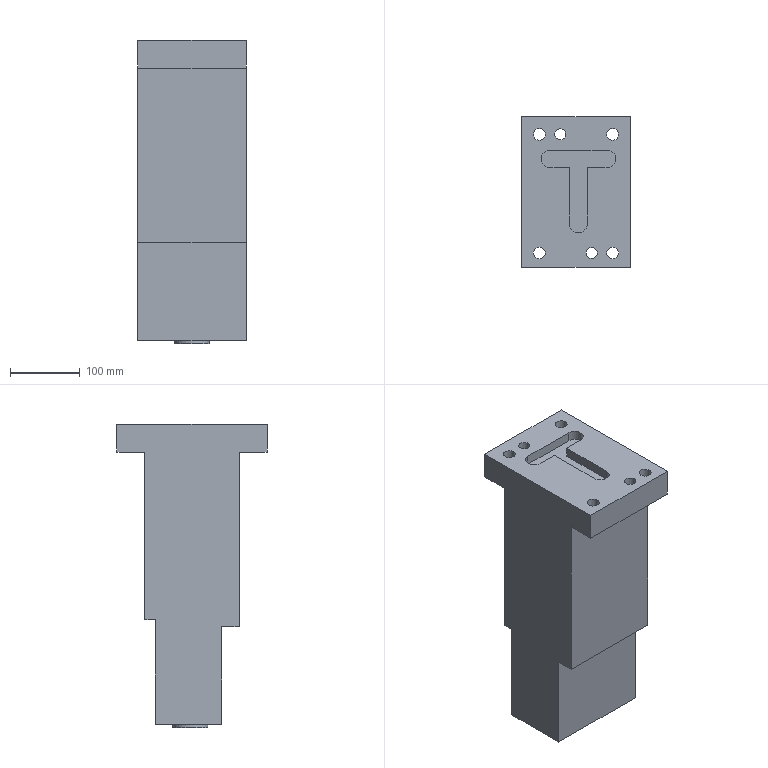Part | NX | features solid 2 | 1 solid | 41 faces | box 155 x 215 x 435 mm | volume 8461392 mm3 | plane 25 | cylinder 15 | cone 1 | commonest cylinder face diameters 25 x7 17 x4 16 x2 20 x1 50 x1
STEP:
#1=CARTESIAN_POINT('',(161.,-435.,130.));
#2=VERTEX_POINT('',#1);
#3=CARTESIAN_POINT('',(169.,-435.,130.));
#4=DIRECTION('',(0.,0.,-1.));
#5=DIRECTION('',(-1.,0.,0.));
#6=AXIS2_PLACEMENT_3D('',#3,#4,#5);
#7=CIRCLE('',#6,8.);
#8=EDGE_CURVE('',#2,#2,#7,.T.);
#9=ORIENTED_EDGE('',*,*,#8,.T.);
#10=EDGE_LOOP('',(#9));
#11=FACE_BOUND('',#10,.T.);
#12=CARTESIAN_POINT('',(206.,-605.,130.));
#13=VERTEX_POINT('',#12);
#14=CARTESIAN_POINT('',(214.,-605.,130.));
#15=DIRECTION('',(0.,0.,-1.));
#16=DIRECTION('',(-1.,0.,0.));
#17=AXIS2_PLACEMENT_3D('',#14,#15,#16);
#18=CIRCLE('',#17,8.);
#19=EDGE_CURVE('',#13,#13,#18,.T.);
#20=ORIENTED_EDGE('',*,*,#19,.T.);
#21=EDGE_LOOP('',(#20));
#22=FACE_BOUND('',#21,.T.);
#23=CARTESIAN_POINT('',(130.5,-435.,130.));
#24=VERTEX_POINT('',#23);
#25=CARTESIAN_POINT('',(139.,-435.,130.));
#26=DIRECTION('',(0.,0.,-1.));
#27=DIRECTION('',(-1.,0.,0.));
#28=AXIS2_PLACEMENT_3D('',#25,#26,#27);
#29=CIRCLE('',#28,8.5);
#30=EDGE_CURVE('',#24,#24,#29,.T.);
#31=ORIENTED_EDGE('',*,*,#30,.T.);
#32=EDGE_LOOP('',(#31));
#33=FACE_BOUND('',#32,.T.);
#34=CARTESIAN_POINT('',(235.5,-435.,130.));
#35=VERTEX_POINT('',#34);
#36=CARTESIAN_POINT('',(244.,-435.,130.));
#37=DIRECTION('',(0.,0.,-1.));
#38=DIRECTION('',(-1.,0.,0.));
#39=AXIS2_PLACEMENT_3D('',#36,#37,#38);
#40=CIRCLE('',#39,8.5);
#41=EDGE_CURVE('',#35,#35,#40,.T.);
#42=ORIENTED_EDGE('',*,*,#41,.T.);
#43=EDGE_LOOP('',(#42));
#44=FACE_BOUND('',#43,.T.);
#45=CARTESIAN_POINT('',(130.5,-605.,130.));
#46=VERTEX_POINT('',#45);
#47=CARTESIAN_POINT('',(139.,-605.,130.));
#48=DIRECTION('',(0.,0.,-1.));
#49=DIRECTION('',(-1.,0.,0.));
#50=AXIS2_PLACEMENT_3D('',#47,#48,#49);
#51=CIRCLE('',#50,8.5);
#52=EDGE_CURVE('',#46,#46,#51,.T.);
#53=ORIENTED_EDGE('',*,*,#52,.T.);
#54=EDGE_LOOP('',(#53));
#55=FACE_BOUND('',#54,.T.);
#56=CARTESIAN_POINT('',(235.5,-605.,130.));
#57=VERTEX_POINT('',#56);
#58=CARTESIAN_POINT('',(244.,-605.,130.));
#59=DIRECTION('',(0.,0.,-1.));
#60=DIRECTION('',(-1.,0.,0.));
#61=AXIS2_PLACEMENT_3D('',#58,#59,#60);
#62=CIRCLE('',#61,8.5);
#63=EDGE_CURVE('',#57,#57,#62,.T.);
#64=ORIENTED_EDGE('',*,*,#63,.T.);
#65=EDGE_LOOP('',(#64));
#66=FACE_BOUND('',#65,.T.);
#67=CARTESIAN_POINT('',(114.,-625.,130.));
#68=VERTEX_POINT('',#67);
#69=CARTESIAN_POINT('',(114.,-410.,130.));
#70=VERTEX_POINT('',#69);
#71=CARTESIAN_POINT('',(114.,-574.335,130.));
#72=DIRECTION('',(0.,1.,0.));
#73=VECTOR('',#72,1000.);
#74=LINE('',#71,#73);
#75=EDGE_CURVE('',#68,#70,#74,.T.);
#76=ORIENTED_EDGE('',*,*,#75,.F.);
#77=CARTESIAN_POINT('',(269.,-625.,130.));
#78=VERTEX_POINT('',#77);
#79=CARTESIAN_POINT('',(106.5,-625.,130.));
#80=DIRECTION('',(1.,0.,0.));
#81=VECTOR('',#80,1000.);
#82=LINE('',#79,#81);
#83=EDGE_CURVE('',#68,#78,#82,.T.);
#84=ORIENTED_EDGE('',*,*,#83,.T.);
#85=CARTESIAN_POINT('',(269.,-410.,130.));
#86=VERTEX_POINT('',#85);
#87=CARTESIAN_POINT('',(269.,-549.335,130.));
#88=DIRECTION('',(0.,1.,0.));
#89=VECTOR('',#88,1000.);
#90=LINE('',#87,#89);
#91=EDGE_CURVE('',#78,#86,#90,.T.);
#92=ORIENTED_EDGE('',*,*,#91,.T.);
#93=CARTESIAN_POINT('',(269.,-410.,130.));
#94=DIRECTION('',(1.,0.,0.));
#95=VECTOR('',#94,1000.);
#96=LINE('',#93,#95);
#97=EDGE_CURVE('',#86,#70,#96,.F.);
#98=ORIENTED_EDGE('',*,*,#97,.T.);
#99=EDGE_LOOP('',(#76,#84,#92,#98));
#100=FACE_BOUND('',#99,.T.);
#101=CARTESIAN_POINT('',(236.,-482.5,130.));
#102=VERTEX_POINT('',#101);
#103=CARTESIAN_POINT('',(207.5,-482.5,130.));
#104=VERTEX_POINT('',#103);
#105=CARTESIAN_POINT('',(106.5,-482.5,130.));
#106=DIRECTION('',(-1.,0.,0.));
#107=VECTOR('',#106,1000.);
#108=LINE('',#105,#107);
#109=EDGE_CURVE('',#102,#104,#108,.T.);
#110=ORIENTED_EDGE('',*,*,#109,.T.);
#111=CARTESIAN_POINT('',(207.5,-563.5,130.));
#112=VERTEX_POINT('',#111);
#113=CARTESIAN_POINT('',(207.5,-574.335,130.));
#114=DIRECTION('',(0.,1.,0.));
#115=VECTOR('',#114,1000.);
#116=LINE('',#113,#115);
#117=EDGE_CURVE('',#112,#104,#116,.T.);
#118=ORIENTED_EDGE('',*,*,#117,.F.);
#119=CARTESIAN_POINT('',(182.5,-563.5,130.));
#120=VERTEX_POINT('',#119);
#121=CARTESIAN_POINT('',(195.,-563.5,130.));
#122=DIRECTION('',(0.,0.,-1.));
#123=DIRECTION('',(1.,0.,0.));
#124=AXIS2_PLACEMENT_3D('',#121,#122,#123);
#125=CIRCLE('',#124,12.5);
#126=EDGE_CURVE('',#112,#120,#125,.T.);
#127=ORIENTED_EDGE('',*,*,#126,.T.);
#128=CARTESIAN_POINT('',(182.5,-482.5,130.));
#129=VERTEX_POINT('',#128);
#130=CARTESIAN_POINT('',(182.5,-574.335,130.));
#131=DIRECTION('',(0.,-1.,0.));
#132=VECTOR('',#131,1000.);
#133=LINE('',#130,#132);
#134=EDGE_CURVE('',#129,#120,#133,.T.);
#135=ORIENTED_EDGE('',*,*,#134,.F.);
#136=CARTESIAN_POINT('',(154.,-482.5,130.));
#137=VERTEX_POINT('',#136);
#138=CARTESIAN_POINT('',(106.5,-482.5,130.));
#139=DIRECTION('',(-1.,0.,0.));
#140=VECTOR('',#139,1000.);
#141=LINE('',#138,#140);
#142=EDGE_CURVE('',#129,#137,#141,.T.);
#143=ORIENTED_EDGE('',*,*,#142,.T.);
#144=CARTESIAN_POINT('',(154.,-457.5,130.));
#145=VERTEX_POINT('',#144);
#146=CARTESIAN_POINT('',(154.,-470.,130.));
#147=DIRECTION('',(0.,0.,-1.));
#148=DIRECTION('',(1.,0.,0.));
#149=AXIS2_PLACEMENT_3D('',#146,#147,#148);
#150=CIRCLE('',#149,12.5);
#151=EDGE_CURVE('',#145,#137,#150,.F.);
#152=ORIENTED_EDGE('',*,*,#151,.F.);
#153=CARTESIAN_POINT('',(236.,-457.5,130.));
#154=VERTEX_POINT('',#153);
#155=CARTESIAN_POINT('',(106.5,-457.5,130.));
#156=DIRECTION('',(-1.,0.,0.));
#157=VECTOR('',#156,1000.);
#158=LINE('',#155,#157);
#159=EDGE_CURVE('',#154,#145,#158,.T.);
#160=ORIENTED_EDGE('',*,*,#159,.F.);
#161=CARTESIAN_POINT('',(236.,-470.,130.));
#162=DIRECTION('',(0.,0.,-1.));
#163=DIRECTION('',(1.,0.,0.));
#164=AXIS2_PLACEMENT_3D('',#161,#162,#163);
#165=CIRCLE('',#164,12.5);
#166=EDGE_CURVE('',#102,#154,#165,.F.);
#167=ORIENTED_EDGE('',*,*,#166,.F.);
#168=EDGE_LOOP('',(#110,#118,#127,#135,#143,#152,#160,#167));
#169=FACE_BOUND('',#168,.T.);
#170=CARTESIAN_POINT('',(106.5,-574.335,130.));
#171=DIRECTION('',(0.,0.,1.));
#172=DIRECTION('',(0.,-1.,0.));
#173=AXIS2_PLACEMENT_3D('',#170,#171,#172);
#174=PLANE('',#173);
#175=ADVANCED_FACE('',(#11,#22,#33,#44,#55,#66,#100,#169),#174,.T.);
#176=CARTESIAN_POINT('',(256.5,-435.,90.));
#177=VERTEX_POINT('',#176);
#178=CARTESIAN_POINT('',(244.,-435.,90.));
#179=DIRECTION('',(0.,0.,1.));
#180=DIRECTION('',(1.,0.,0.));
#181=AXIS2_PLACEMENT_3D('',#178,#179,#180);
#182=CIRCLE('',#181,12.5);
#183=EDGE_CURVE('',#177,#177,#182,.T.);
#184=ORIENTED_EDGE('',*,*,#183,.T.);
#185=EDGE_LOOP('',(#184));
#186=FACE_BOUND('',#185,.T.);
#187=CARTESIAN_POINT('',(151.5,-435.,90.));
#188=VERTEX_POINT('',#187);
#189=CARTESIAN_POINT('',(139.,-435.,90.));
#190=DIRECTION('',(0.,0.,1.));
#191=DIRECTION('',(1.,0.,0.));
#192=AXIS2_PLACEMENT_3D('',#189,#190,#191);
#193=CIRCLE('',#192,12.5);
#194=EDGE_CURVE('',#188,#188,#193,.F.);
#195=ORIENTED_EDGE('',*,*,#194,.F.);
#196=EDGE_LOOP('',(#195));
#197=FACE_BOUND('',#196,.T.);
#198=CARTESIAN_POINT('',(177.,-435.,90.));
#199=VERTEX_POINT('',#198);
#200=CARTESIAN_POINT('',(169.,-435.,90.));
#201=DIRECTION('',(0.,0.,1.));
#202=DIRECTION('',(1.,0.,0.));
#203=AXIS2_PLACEMENT_3D('',#200,#201,#202);
#204=CIRCLE('',#203,8.);
#205=EDGE_CURVE('',#199,#199,#204,.F.);
#206=ORIENTED_EDGE('',*,*,#205,.F.);
#207=EDGE_LOOP('',(#206));
#208=FACE_BOUND('',#207,.T.);
#209=CARTESIAN_POINT('',(269.,-450.,90.));
#210=VERTEX_POINT('',#209);
#211=CARTESIAN_POINT('',(114.,-450.,90.));
#212=VERTEX_POINT('',#211);
#213=CARTESIAN_POINT('',(849.,-450.,90.));
#214=DIRECTION('',(-1.,0.,0.));
#215=VECTOR('',#214,1000.);
#216=LINE('',#213,#215);
#217=EDGE_CURVE('',#210,#212,#216,.T.);
#218=ORIENTED_EDGE('',*,*,#217,.T.);
#219=CARTESIAN_POINT('',(114.,-410.,90.));
#220=VERTEX_POINT('',#219);
#221=CARTESIAN_POINT('',(114.,-494.335,90.));
#222=DIRECTION('',(0.,-1.,0.));
#223=VECTOR('',#222,1000.);
#224=LINE('',#221,#223);
#225=EDGE_CURVE('',#212,#220,#224,.F.);
#226=ORIENTED_EDGE('',*,*,#225,.T.);
#227=CARTESIAN_POINT('',(269.,-410.,90.));
#228=VERTEX_POINT('',#227);
#229=CARTESIAN_POINT('',(269.,-410.,90.));
#230=DIRECTION('',(-1.,0.,0.));
#231=VECTOR('',#230,1000.);
#232=LINE('',#229,#231);
#233=EDGE_CURVE('',#228,#220,#232,.T.);
#234=ORIENTED_EDGE('',*,*,#233,.F.);
#235=CARTESIAN_POINT('',(269.,-549.335,90.));
#236=DIRECTION('',(0.,-1.,0.));
#237=VECTOR('',#236,1000.);
#238=LINE('',#235,#237);
#239=EDGE_CURVE('',#210,#228,#238,.F.);
#240=ORIENTED_EDGE('',*,*,#239,.F.);
#241=EDGE_LOOP('',(#218,#226,#234,#240));
#242=FACE_BOUND('',#241,.T.);
#243=CARTESIAN_POINT('',(269.,-494.335,90.));
#244=DIRECTION('',(0.,0.,-1.));
#245=DIRECTION('',(-1.,0.,0.));
#246=AXIS2_PLACEMENT_3D('',#243,#244,#245);
#247=PLANE('',#246);
#248=ADVANCED_FACE('',(#186,#197,#208,#242),#247,.T.);
#249=CARTESIAN_POINT('',(256.5,-605.,90.));
#250=VERTEX_POINT('',#249);
#251=CARTESIAN_POINT('',(244.,-605.,90.));
#252=DIRECTION('',(0.,0.,1.));
#253=DIRECTION('',(1.,0.,0.));
#254=AXIS2_PLACEMENT_3D('',#251,#252,#253);
#255=CIRCLE('',#254,12.5);
#256=EDGE_CURVE('',#250,#250,#255,.F.);
#257=ORIENTED_EDGE('',*,*,#256,.F.);
#258=EDGE_LOOP('',(#257));
#259=FACE_BOUND('',#258,.T.);
#260=CARTESIAN_POINT('',(151.5,-605.,90.));
#261=VERTEX_POINT('',#260);
#262=CARTESIAN_POINT('',(139.,-605.,90.));
#263=DIRECTION('',(0.,0.,1.));
#264=DIRECTION('',(1.,0.,0.));
#265=AXIS2_PLACEMENT_3D('',#262,#263,#264);
#266=CIRCLE('',#265,12.5);
#267=EDGE_CURVE('',#261,#261,#266,.F.);
#268=ORIENTED_EDGE('',*,*,#267,.F.);
#269=EDGE_LOOP('',(#268));
#270=FACE_BOUND('',#269,.T.);
#271=CARTESIAN_POINT('',(222.,-605.,90.));
#272=VERTEX_POINT('',#271);
#273=CARTESIAN_POINT('',(214.,-605.,90.));
#274=DIRECTION('',(0.,0.,1.));
#275=DIRECTION('',(1.,0.,0.));
#276=AXIS2_PLACEMENT_3D('',#273,#274,#275);
#277=CIRCLE('',#276,8.);
#278=EDGE_CURVE('',#272,#272,#277,.F.);
#279=ORIENTED_EDGE('',*,*,#278,.F.);
#280=EDGE_LOOP('',(#279));
#281=FACE_BOUND('',#280,.T.);
#282=CARTESIAN_POINT('',(114.,-585.,90.));
#283=VERTEX_POINT('',#282);
#284=CARTESIAN_POINT('',(269.,-585.,90.));
#285=VERTEX_POINT('',#284);
#286=CARTESIAN_POINT('',(269.,-585.,90.));
#287=DIRECTION('',(1.,0.,0.));
#288=VECTOR('',#287,1000.);
#289=LINE('',#286,#288);
#290=EDGE_CURVE('',#283,#285,#289,.T.);
#291=ORIENTED_EDGE('',*,*,#290,.T.);
#292=CARTESIAN_POINT('',(269.,-625.,90.));
#293=VERTEX_POINT('',#292);
#294=CARTESIAN_POINT('',(269.,-489.335,90.));
#295=DIRECTION('',(0.,1.,0.));
#296=VECTOR('',#295,1000.);
#297=LINE('',#294,#296);
#298=EDGE_CURVE('',#285,#293,#297,.F.);
#299=ORIENTED_EDGE('',*,*,#298,.T.);
#300=CARTESIAN_POINT('',(114.,-625.,90.));
#301=VERTEX_POINT('',#300);
#302=CARTESIAN_POINT('',(269.,-625.,90.));
#303=DIRECTION('',(-1.,0.,0.));
#304=VECTOR('',#303,1000.);
#305=LINE('',#302,#304);
#306=EDGE_CURVE('',#301,#293,#305,.F.);
#307=ORIENTED_EDGE('',*,*,#306,.F.);
#308=CARTESIAN_POINT('',(114.,-489.335,90.));
#309=DIRECTION('',(0.,-1.,0.));
#310=VECTOR('',#309,1000.);
#311=LINE('',#308,#310);
#312=EDGE_CURVE('',#301,#283,#311,.F.);
#313=ORIENTED_EDGE('',*,*,#312,.T.);
#314=EDGE_LOOP('',(#291,#299,#307,#313));
#315=FACE_BOUND('',#314,.T.);
#316=CARTESIAN_POINT('',(269.,-489.335,90.));
#317=DIRECTION('',(0.,0.,-1.));
#318=DIRECTION('',(-1.,0.,0.));
#319=AXIS2_PLACEMENT_3D('',#316,#317,#318);
#320=PLANE('',#319);
#321=ADVANCED_FACE('',(#259,#270,#281,#315),#320,.T.);
#322=ORIENTED_EDGE('',*,*,#312,.F.);
#323=CARTESIAN_POINT('',(114.,-625.,215.));
#324=DIRECTION('',(0.,0.,-1.));
#325=VECTOR('',#324,1000.);
#326=LINE('',#323,#325);
#327=EDGE_CURVE('',#68,#301,#326,.T.);
#328=ORIENTED_EDGE('',*,*,#327,.F.);
#329=ORIENTED_EDGE('',*,*,#75,.T.);
#330=CARTESIAN_POINT('',(114.,-410.,190.));
#331=DIRECTION('',(0.,0.,1.));
#332=VECTOR('',#331,1000.);
#333=LINE('',#330,#332);
#334=EDGE_CURVE('',#220,#70,#333,.T.);
#335=ORIENTED_EDGE('',*,*,#334,.F.);
#336=ORIENTED_EDGE('',*,*,#225,.F.);
#337=CARTESIAN_POINT('',(114.,-450.,-150.));
#338=VERTEX_POINT('',#337);
#339=CARTESIAN_POINT('',(114.,-450.,-43.));
#340=DIRECTION('',(0.,0.,-1.));
#341=VECTOR('',#340,1000.);
#342=LINE('',#339,#341);
#343=EDGE_CURVE('',#212,#338,#342,.T.);
#344=ORIENTED_EDGE('',*,*,#343,.T.);
#345=CARTESIAN_POINT('',(114.,-465.,-150.));
#346=VERTEX_POINT('',#345);
#347=CARTESIAN_POINT('',(114.,-559.335,-150.));
#348=DIRECTION('',(0.,1.,0.));
#349=VECTOR('',#348,1000.);
#350=LINE('',#347,#349);
#351=EDGE_CURVE('',#338,#346,#350,.F.);
#352=ORIENTED_EDGE('',*,*,#351,.T.);
#353=CARTESIAN_POINT('',(114.,-465.,-300.));
#354=VERTEX_POINT('',#353);
#355=CARTESIAN_POINT('',(114.,-465.,10.));
#356=DIRECTION('',(0.,0.,-1.));
#357=VECTOR('',#356,1000.);
#358=LINE('',#355,#357);
#359=EDGE_CURVE('',#346,#354,#358,.T.);
#360=ORIENTED_EDGE('',*,*,#359,.T.);
#361=CARTESIAN_POINT('',(114.,-560.,-300.));
#362=VERTEX_POINT('',#361);
#363=CARTESIAN_POINT('',(114.,-574.793,-300.));
#364=DIRECTION('',(0.,-1.,0.));
#365=VECTOR('',#364,1000.);
#366=LINE('',#363,#365);
#367=EDGE_CURVE('',#354,#362,#366,.T.);
#368=ORIENTED_EDGE('',*,*,#367,.T.);
#369=CARTESIAN_POINT('',(114.,-560.,-160.));
#370=VERTEX_POINT('',#369);
#371=CARTESIAN_POINT('',(114.,-560.,-105.));
#372=DIRECTION('',(0.,0.,-1.));
#373=VECTOR('',#372,1000.);
#374=LINE('',#371,#373);
#375=EDGE_CURVE('',#370,#362,#374,.T.);
#376=ORIENTED_EDGE('',*,*,#375,.F.);
#377=CARTESIAN_POINT('',(114.,-585.,-160.));
#378=VERTEX_POINT('',#377);
#379=CARTESIAN_POINT('',(114.,-564.335,-160.));
#380=DIRECTION('',(0.,1.,0.));
#381=VECTOR('',#380,1000.);
#382=LINE('',#379,#381);
#383=EDGE_CURVE('',#370,#378,#382,.F.);
#384=ORIENTED_EDGE('',*,*,#383,.T.);
#385=CARTESIAN_POINT('',(114.,-585.,-110.));
#386=DIRECTION('',(0.,0.,-1.));
#387=VECTOR('',#386,1000.);
#388=LINE('',#385,#387);
#389=EDGE_CURVE('',#378,#283,#388,.F.);
#390=ORIENTED_EDGE('',*,*,#389,.T.);
#391=EDGE_LOOP('',(#322,#328,#329,#335,#336,#344,#352,#360,#368,#376,#384,#390));
#392=FACE_BOUND('',#391,.T.);
#393=CARTESIAN_POINT('',(114.,-559.335,-105.));
#394=DIRECTION('',(-1.,0.,0.));
#395=DIRECTION('',(0.,1.,0.));
#396=AXIS2_PLACEMENT_3D('',#393,#394,#395);
#397=PLANE('',#396);
#398=ADVANCED_FACE('',(#392),#397,.T.);
#399=ORIENTED_EDGE('',*,*,#91,.F.);
#400=CARTESIAN_POINT('',(269.,-625.,215.));
#401=DIRECTION('',(0.,0.,1.));
#402=VECTOR('',#401,1000.);
#403=LINE('',#400,#402);
#404=EDGE_CURVE('',#293,#78,#403,.T.);
#405=ORIENTED_EDGE('',*,*,#404,.F.);
#406=ORIENTED_EDGE('',*,*,#298,.F.);
#407=CARTESIAN_POINT('',(269.,-585.,-160.));
#408=VERTEX_POINT('',#407);
#409=CARTESIAN_POINT('',(269.,-585.,-40.));
#410=DIRECTION('',(0.,0.,-1.));
#411=VECTOR('',#410,1000.);
#412=LINE('',#409,#411);
#413=EDGE_CURVE('',#408,#285,#412,.F.);
#414=ORIENTED_EDGE('',*,*,#413,.F.);
#415=CARTESIAN_POINT('',(269.,-560.,-160.));
#416=VERTEX_POINT('',#415);
#417=CARTESIAN_POINT('',(269.,-549.335,-160.));
#418=DIRECTION('',(0.,1.,0.));
#419=VECTOR('',#418,1000.);
#420=LINE('',#417,#419);
#421=EDGE_CURVE('',#416,#408,#420,.F.);
#422=ORIENTED_EDGE('',*,*,#421,.F.);
#423=CARTESIAN_POINT('',(269.,-560.,-300.));
#424=VERTEX_POINT('',#423);
#425=CARTESIAN_POINT('',(269.,-560.,-50.));
#426=DIRECTION('',(0.,0.,-1.));
#427=VECTOR('',#426,1000.);
#428=LINE('',#425,#427);
#429=EDGE_CURVE('',#416,#424,#428,.T.);
#430=ORIENTED_EDGE('',*,*,#429,.T.);
#431=CARTESIAN_POINT('',(269.,-465.,-300.));
#432=VERTEX_POINT('',#431);
#433=CARTESIAN_POINT('',(269.,-549.335,-300.));
#434=DIRECTION('',(0.,-1.,0.));
#435=VECTOR('',#434,1000.);
#436=LINE('',#433,#435);
#437=EDGE_CURVE('',#432,#424,#436,.T.);
#438=ORIENTED_EDGE('',*,*,#437,.F.);
#439=CARTESIAN_POINT('',(269.,-465.,-150.));
#440=VERTEX_POINT('',#439);
#441=CARTESIAN_POINT('',(269.,-465.,-105.));
#442=DIRECTION('',(0.,0.,-1.));
#443=VECTOR('',#442,1000.);
#444=LINE('',#441,#443);
#445=EDGE_CURVE('',#440,#432,#444,.T.);
#446=ORIENTED_EDGE('',*,*,#445,.F.);
#447=CARTESIAN_POINT('',(269.,-450.,-150.));
#448=VERTEX_POINT('',#447);
#449=CARTESIAN_POINT('',(269.,-455.,-150.));
#450=DIRECTION('',(0.,1.,0.));
#451=VECTOR('',#450,1000.);
#452=LINE('',#449,#451);
#453=EDGE_CURVE('',#448,#440,#452,.F.);
#454=ORIENTED_EDGE('',*,*,#453,.F.);
#455=CARTESIAN_POINT('',(269.,-450.,-105.));
#456=DIRECTION('',(0.,0.,-1.));
#457=VECTOR('',#456,1000.);
#458=LINE('',#455,#457);
#459=EDGE_CURVE('',#210,#448,#458,.T.);
#460=ORIENTED_EDGE('',*,*,#459,.F.);
#461=ORIENTED_EDGE('',*,*,#239,.T.);
#462=CARTESIAN_POINT('',(269.,-410.,-105.));
#463=DIRECTION('',(0.,0.,1.));
#464=VECTOR('',#463,1000.);
#465=LINE('',#462,#464);
#466=EDGE_CURVE('',#86,#228,#465,.F.);
#467=ORIENTED_EDGE('',*,*,#466,.F.);
#468=EDGE_LOOP('',(#399,#405,#406,#414,#422,#430,#438,#446,#454,#460,#461,#467));
#469=FACE_BOUND('',#468,.T.);
#470=CARTESIAN_POINT('',(269.,-549.335,-105.));
#471=DIRECTION('',(1.,0.,0.));
#472=DIRECTION('',(0.,-1.,0.));
#473=AXIS2_PLACEMENT_3D('',#470,#471,#472);
#474=PLANE('',#473);
#475=ADVANCED_FACE('',(#469),#474,.T.);
#476=ORIENTED_EDGE('',*,*,#404,.T.);
#477=ORIENTED_EDGE('',*,*,#83,.F.);
#478=ORIENTED_EDGE('',*,*,#327,.T.);
#479=ORIENTED_EDGE('',*,*,#306,.T.);
#480=EDGE_LOOP('',(#476,#477,#478,#479));
#481=FACE_BOUND('',#480,.T.);
#482=CARTESIAN_POINT('',(106.5,-625.,115.));
#483=DIRECTION('',(0.,1.,0.));
#484=DIRECTION('',(0.,0.,-1.));
#485=AXIS2_PLACEMENT_3D('',#482,#483,#484);
#486=PLANE('',#485);
#487=ADVANCED_FACE('',(#481),#486,.F.);
#488=ORIENTED_EDGE('',*,*,#233,.T.);
#489=ORIENTED_EDGE('',*,*,#334,.T.);
#490=ORIENTED_EDGE('',*,*,#97,.F.);
#491=ORIENTED_EDGE('',*,*,#466,.T.);
#492=EDGE_LOOP('',(#488,#489,#490,#491));
#493=FACE_BOUND('',#492,.T.);
#494=CARTESIAN_POINT('',(269.,-410.,90.));
#495=DIRECTION('',(0.,-1.,0.));
#496=DIRECTION('',(0.,0.,-1.));
#497=AXIS2_PLACEMENT_3D('',#494,#495,#496);
#498=PLANE('',#497);
#499=ADVANCED_FACE('',(#493),#498,.F.);
#500=ORIENTED_EDGE('',*,*,#63,.F.);
#501=EDGE_LOOP('',(#500));
#502=FACE_BOUND('',#501,.T.);
#503=CARTESIAN_POINT('',(252.5,-605.,110.));
#504=VERTEX_POINT('',#503);
#505=CARTESIAN_POINT('',(244.,-605.,110.));
#506=DIRECTION('',(0.,0.,-1.));
#507=DIRECTION('',(1.,0.,0.));
#508=AXIS2_PLACEMENT_3D('',#505,#506,#507);
#509=CIRCLE('',#508,8.5);
#510=EDGE_CURVE('',#504,#504,#509,.T.);
#511=ORIENTED_EDGE('',*,*,#510,.T.);
#512=EDGE_LOOP('',(#511));
#513=FACE_BOUND('',#512,.T.);
#514=CARTESIAN_POINT('',(244.,-605.,130.));
#515=DIRECTION('',(0.,0.,1.));
#516=DIRECTION('',(-1.,0.,0.));
#517=AXIS2_PLACEMENT_3D('',#514,#515,#516);
#518=CYLINDRICAL_SURFACE('',#517,8.5);
#519=ADVANCED_FACE('',(#502,#513),#518,.F.);
#520=ORIENTED_EDGE('',*,*,#510,.F.);
#521=EDGE_LOOP('',(#520));
#522=FACE_BOUND('',#521,.T.);
#523=CARTESIAN_POINT('',(256.5,-605.,110.));
#524=VERTEX_POINT('',#523);
#525=CARTESIAN_POINT('',(244.,-605.,110.));
#526=DIRECTION('',(0.,0.,-1.));
#527=DIRECTION('',(1.,0.,0.));
#528=AXIS2_PLACEMENT_3D('',#525,#526,#527);
#529=CIRCLE('',#528,12.5);
#530=EDGE_CURVE('',#524,#524,#529,.T.);
#531=ORIENTED_EDGE('',*,*,#530,.T.);
#532=EDGE_LOOP('',(#531));
#533=FACE_BOUND('',#532,.T.);
#534=CARTESIAN_POINT('',(139.,-435.,110.));
#535=DIRECTION('',(0.,0.,1.));
#536=DIRECTION('',(-1.,0.,0.));
#537=AXIS2_PLACEMENT_3D('',#534,#535,#536);
#538=PLANE('',#537);
#539=ADVANCED_FACE('',(#522,#533),#538,.F.);
#540=ORIENTED_EDGE('',*,*,#530,.F.);
#541=EDGE_LOOP('',(#540));
#542=FACE_BOUND('',#541,.T.);
#543=ORIENTED_EDGE('',*,*,#256,.T.);
#544=EDGE_LOOP('',(#543));
#545=FACE_BOUND('',#544,.T.);
#546=CARTESIAN_POINT('',(244.,-605.,80.));
#547=DIRECTION('',(0.,0.,1.));
#548=DIRECTION('',(-1.,0.,0.));
#549=AXIS2_PLACEMENT_3D('',#546,#547,#548);
#550=CYLINDRICAL_SURFACE('',#549,12.5);
#551=ADVANCED_FACE('',(#542,#545),#550,.F.);
#552=ORIENTED_EDGE('',*,*,#52,.F.);
#553=EDGE_LOOP('',(#552));
#554=FACE_BOUND('',#553,.T.);
#555=CARTESIAN_POINT('',(147.5,-605.,110.));
#556=VERTEX_POINT('',#555);
#557=CARTESIAN_POINT('',(139.,-605.,110.));
#558=DIRECTION('',(0.,0.,-1.));
#559=DIRECTION('',(1.,0.,0.));
#560=AXIS2_PLACEMENT_3D('',#557,#558,#559);
#561=CIRCLE('',#560,8.5);
#562=EDGE_CURVE('',#556,#556,#561,.T.);
#563=ORIENTED_EDGE('',*,*,#562,.T.);
#564=EDGE_LOOP('',(#563));
#565=FACE_BOUND('',#564,.T.);
#566=CARTESIAN_POINT('',(139.,-605.,130.));
#567=DIRECTION('',(0.,0.,1.));
#568=DIRECTION('',(-1.,0.,0.));
#569=AXIS2_PLACEMENT_3D('',#566,#567,#568);
#570=CYLINDRICAL_SURFACE('',#569,8.5);
#571=ADVANCED_FACE('',(#554,#565),#570,.F.);
#572=ORIENTED_EDGE('',*,*,#562,.F.);
#573=EDGE_LOOP('',(#572));
#574=FACE_BOUND('',#573,.T.);
#575=CARTESIAN_POINT('',(151.5,-605.,110.));
#576=VERTEX_POINT('',#575);
#577=CARTESIAN_POINT('',(139.,-605.,110.));
#578=DIRECTION('',(0.,0.,-1.));
#579=DIRECTION('',(1.,0.,0.));
#580=AXIS2_PLACEMENT_3D('',#577,#578,#579);
#581=CIRCLE('',#580,12.5);
#582=EDGE_CURVE('',#576,#576,#581,.T.);
#583=ORIENTED_EDGE('',*,*,#582,.T.);
#584=EDGE_LOOP('',(#583));
#585=FACE_BOUND('',#584,.T.);
#586=CARTESIAN_POINT('',(139.,-435.,110.));
#587=DIRECTION('',(0.,0.,1.));
#588=DIRECTION('',(-1.,0.,0.));
#589=AXIS2_PLACEMENT_3D('',#586,#587,#588);
#590=PLANE('',#589);
#591=ADVANCED_FACE('',(#574,#585),#590,.F.);
#592=ORIENTED_EDGE('',*,*,#582,.F.);
#593=EDGE_LOOP('',(#592));
#594=FACE_BOUND('',#593,.T.);
#595=ORIENTED_EDGE('',*,*,#267,.T.);
#596=EDGE_LOOP('',(#595));
#597=FACE_BOUND('',#596,.T.);
#598=CARTESIAN_POINT('',(139.,-605.,80.));
#599=DIRECTION('',(0.,0.,1.));
#600=DIRECTION('',(-1.,0.,0.));
#601=AXIS2_PLACEMENT_3D('',#598,#599,#600);
#602=CYLINDRICAL_SURFACE('',#601,12.5);
#603=ADVANCED_FACE('',(#594,#597),#602,.F.);
#604=ORIENTED_EDGE('',*,*,#41,.F.);
#605=EDGE_LOOP('',(#604));
#606=FACE_BOUND('',#605,.T.);
#607=CARTESIAN_POINT('',(252.5,-435.,110.));
#608=VERTEX_POINT('',#607);
#609=CARTESIAN_POINT('',(244.,-435.,110.));
#610=DIRECTION('',(0.,0.,-1.));
#611=DIRECTION('',(1.,0.,0.));
#612=AXIS2_PLACEMENT_3D('',#609,#610,#611);
#613=CIRCLE('',#612,8.5);
#614=EDGE_CURVE('',#608,#608,#613,.T.);
#615=ORIENTED_EDGE('',*,*,#614,.T.);
#616=EDGE_LOOP('',(#615));
#617=FACE_BOUND('',#616,.T.);
#618=CARTESIAN_POINT('',(244.,-435.,140.));
#619=DIRECTION('',(0.,0.,1.));
#620=DIRECTION('',(-1.,0.,0.));
#621=AXIS2_PLACEMENT_3D('',#618,#619,#620);
#622=CYLINDRICAL_SURFACE('',#621,8.5);
#623=ADVANCED_FACE('',(#606,#617),#622,.F.);
#624=ORIENTED_EDGE('',*,*,#614,.F.);
#625=EDGE_LOOP('',(#624));
#626=FACE_BOUND('',#625,.T.);
#627=CARTESIAN_POINT('',(256.5,-435.,110.));
#628=VERTEX_POINT('',#627);
#629=CARTESIAN_POINT('',(244.,-435.,110.));
#630=DIRECTION('',(0.,0.,-1.));
#631=DIRECTION('',(1.,0.,0.));
#632=AXIS2_PLACEMENT_3D('',#629,#630,#631);
#633=CIRCLE('',#632,12.5);
#634=EDGE_CURVE('',#628,#628,#633,.T.);
#635=ORIENTED_EDGE('',*,*,#634,.T.);
#636=EDGE_LOOP('',(#635));
#637=FACE_BOUND('',#636,.T.);
#638=CARTESIAN_POINT('',(139.,-435.,110.));
#639=DIRECTION('',(0.,0.,1.));
#640=DIRECTION('',(-1.,0.,0.));
#641=AXIS2_PLACEMENT_3D('',#638,#639,#640);
#642=PLANE('',#641);
#643=ADVANCED_FACE('',(#626,#637),#642,.F.);
#644=ORIENTED_EDGE('',*,*,#634,.F.);
#645=EDGE_LOOP('',(#644));
#646=FACE_BOUND('',#645,.T.);
#647=ORIENTED_EDGE('',*,*,#183,.F.);
#648=EDGE_LOOP('',(#647));
#649=FACE_BOUND('',#648,.T.);
#650=CARTESIAN_POINT('',(244.,-435.,90.));
#651=DIRECTION('',(0.,0.,1.));
#652=DIRECTION('',(-1.,0.,0.));
#653=AXIS2_PLACEMENT_3D('',#650,#651,#652);
#654=CYLINDRICAL_SURFACE('',#653,12.5);
#655=ADVANCED_FACE('',(#646,#649),#654,.F.);
#656=ORIENTED_EDGE('',*,*,#30,.F.);
#657=EDGE_LOOP('',(#656));
#658=FACE_BOUND('',#657,.T.);
#659=CARTESIAN_POINT('',(130.5,-435.,110.));
#660=VERTEX_POINT('',#659);
#661=CARTESIAN_POINT('',(139.,-435.,110.));
#662=DIRECTION('',(0.,0.,-1.));
#663=DIRECTION('',(-1.,0.,0.));
#664=AXIS2_PLACEMENT_3D('',#661,#662,#663);
#665=CIRCLE('',#664,8.5);
#666=EDGE_CURVE('',#660,#660,#665,.T.);
#667=ORIENTED_EDGE('',*,*,#666,.T.);
#668=EDGE_LOOP('',(#667));
#669=FACE_BOUND('',#668,.T.);
#670=CARTESIAN_POINT('',(139.,-435.,140.));
#671=DIRECTION('',(0.,0.,1.));
#672=DIRECTION('',(-1.,0.,0.));
#673=AXIS2_PLACEMENT_3D('',#670,#671,#672);
#674=CYLINDRICAL_SURFACE('',#673,8.5);
#675=ADVANCED_FACE('',(#658,#669),#674,.F.);
#676=ORIENTED_EDGE('',*,*,#666,.F.);
#677=EDGE_LOOP('',(#676));
#678=FACE_BOUND('',#677,.T.);
#679=CARTESIAN_POINT('',(126.5,-435.,110.));
#680=VERTEX_POINT('',#679);
#681=CARTESIAN_POINT('',(139.,-435.,110.));
#682=DIRECTION('',(0.,0.,-1.));
#683=DIRECTION('',(-1.,0.,0.));
#684=AXIS2_PLACEMENT_3D('',#681,#682,#683);
#685=CIRCLE('',#684,12.5);
#686=EDGE_CURVE('',#680,#680,#685,.T.);
#687=ORIENTED_EDGE('',*,*,#686,.T.);
#688=EDGE_LOOP('',(#687));
#689=FACE_BOUND('',#688,.T.);
#690=CARTESIAN_POINT('',(139.,-435.,110.));
#691=DIRECTION('',(0.,0.,1.));
#692=DIRECTION('',(-1.,0.,0.));
#693=AXIS2_PLACEMENT_3D('',#690,#691,#692);
#694=PLANE('',#693);
#695=ADVANCED_FACE('',(#678,#689),#694,.F.);
#696=ORIENTED_EDGE('',*,*,#686,.F.);
#697=EDGE_LOOP('',(#696));
#698=FACE_BOUND('',#697,.T.);
#699=ORIENTED_EDGE('',*,*,#194,.T.);
#700=EDGE_LOOP('',(#699));
#701=FACE_BOUND('',#700,.T.);
#702=CARTESIAN_POINT('',(139.,-435.,90.));
#703=DIRECTION('',(0.,0.,1.));
#704=DIRECTION('',(-1.,0.,0.));
#705=AXIS2_PLACEMENT_3D('',#702,#703,#704);
#706=CYLINDRICAL_SURFACE('',#705,12.5);
#707=ADVANCED_FACE('',(#698,#701),#706,.F.);
#708=ORIENTED_EDGE('',*,*,#19,.F.);
#709=EDGE_LOOP('',(#708));
#710=FACE_BOUND('',#709,.T.);
#711=ORIENTED_EDGE('',*,*,#278,.T.);
#712=EDGE_LOOP('',(#711));
#713=FACE_BOUND('',#712,.T.);
#714=CARTESIAN_POINT('',(214.,-605.,80.));
#715=DIRECTION('',(0.,0.,1.));
#716=DIRECTION('',(-1.,0.,0.));
#717=AXIS2_PLACEMENT_3D('',#714,#715,#716);
#718=CYLINDRICAL_SURFACE('',#717,8.);
#719=ADVANCED_FACE('',(#710,#713),#718,.F.);
#720=ORIENTED_EDGE('',*,*,#8,.F.);
#721=EDGE_LOOP('',(#720));
#722=FACE_BOUND('',#721,.T.);
#723=ORIENTED_EDGE('',*,*,#205,.T.);
#724=EDGE_LOOP('',(#723));
#725=FACE_BOUND('',#724,.T.);
#726=CARTESIAN_POINT('',(169.,-435.,90.));
#727=DIRECTION('',(0.,0.,1.));
#728=DIRECTION('',(-1.,0.,0.));
#729=AXIS2_PLACEMENT_3D('',#726,#727,#728);
#730=CYLINDRICAL_SURFACE('',#729,8.);
#731=ADVANCED_FACE('',(#722,#725),#730,.F.);
#732=ORIENTED_EDGE('',*,*,#459,.T.);
#733=CARTESIAN_POINT('',(229.,-450.,-150.));
#734=DIRECTION('',(-1.,0.,0.));
#735=VECTOR('',#734,1000.);
#736=LINE('',#733,#735);
#737=EDGE_CURVE('',#338,#448,#736,.F.);
#738=ORIENTED_EDGE('',*,*,#737,.F.);
#739=ORIENTED_EDGE('',*,*,#343,.F.);
#740=ORIENTED_EDGE('',*,*,#217,.F.);
#741=EDGE_LOOP('',(#732,#738,#739,#740));
#742=FACE_BOUND('',#741,.T.);
#743=CARTESIAN_POINT('',(688.5,-450.,-143.));
#744=DIRECTION('',(0.,1.,0.));
#745=DIRECTION('',(1.,0.,0.));
#746=AXIS2_PLACEMENT_3D('',#743,#744,#745);
#747=PLANE('',#746);
#748=ADVANCED_FACE('',(#742),#747,.T.);
#749=CARTESIAN_POINT('',(166.5,-515.,-300.));
#750=VERTEX_POINT('',#749);
#751=CARTESIAN_POINT('',(191.5,-515.,-300.));
#752=DIRECTION('',(0.,0.,1.));
#753=DIRECTION('',(-1.,0.,0.));
#754=AXIS2_PLACEMENT_3D('',#751,#752,#753);
#755=CIRCLE('',#754,25.);
#756=EDGE_CURVE('',#750,#750,#755,.T.);
#757=ORIENTED_EDGE('',*,*,#756,.T.);
#758=EDGE_LOOP('',(#757));
#759=FACE_BOUND('',#758,.T.);
#760=CARTESIAN_POINT('',(229.,-560.,-300.));
#761=DIRECTION('',(1.,0.,0.));
#762=VECTOR('',#761,1000.);
#763=LINE('',#760,#762);
#764=EDGE_CURVE('',#362,#424,#763,.T.);
#765=ORIENTED_EDGE('',*,*,#764,.F.);
#766=ORIENTED_EDGE('',*,*,#367,.F.);
#767=CARTESIAN_POINT('',(382.,-465.,-300.));
#768=DIRECTION('',(1.,0.,0.));
#769=VECTOR('',#768,1000.);
#770=LINE('',#767,#769);
#771=EDGE_CURVE('',#354,#432,#770,.T.);
#772=ORIENTED_EDGE('',*,*,#771,.T.);
#773=ORIENTED_EDGE('',*,*,#437,.T.);
#774=EDGE_LOOP('',(#765,#766,#772,#773));
#775=FACE_BOUND('',#774,.T.);
#776=CARTESIAN_POINT('',(229.,-574.793,-300.));
#777=DIRECTION('',(0.,0.,-1.));
#778=DIRECTION('',(-1.,0.,0.));
#779=AXIS2_PLACEMENT_3D('',#776,#777,#778);
#780=PLANE('',#779);
#781=ADVANCED_FACE('',(#759,#775),#780,.T.);
#782=ORIENTED_EDGE('',*,*,#290,.F.);
#783=ORIENTED_EDGE('',*,*,#389,.F.);
#784=CARTESIAN_POINT('',(686.5,-585.,-160.));
#785=DIRECTION('',(1.,0.,0.));
#786=VECTOR('',#785,1000.);
#787=LINE('',#784,#786);
#788=EDGE_CURVE('',#378,#408,#787,.T.);
#789=ORIENTED_EDGE('',*,*,#788,.T.);
#790=ORIENTED_EDGE('',*,*,#413,.T.);
#791=EDGE_LOOP('',(#782,#783,#789,#790));
#792=FACE_BOUND('',#791,.T.);
#793=CARTESIAN_POINT('',(686.5,-585.,-140.));
#794=DIRECTION('',(0.,-1.,0.));
#795=DIRECTION('',(1.,0.,0.));
#796=AXIS2_PLACEMENT_3D('',#793,#794,#795);
#797=PLANE('',#796);
#798=ADVANCED_FACE('',(#792),#797,.T.);
#799=ORIENTED_EDGE('',*,*,#453,.T.);
#800=CARTESIAN_POINT('',(229.,-465.,-150.));
#801=DIRECTION('',(-1.,0.,0.));
#802=VECTOR('',#801,1000.);
#803=LINE('',#800,#802);
#804=EDGE_CURVE('',#346,#440,#803,.F.);
#805=ORIENTED_EDGE('',*,*,#804,.F.);
#806=ORIENTED_EDGE('',*,*,#351,.F.);
#807=ORIENTED_EDGE('',*,*,#737,.T.);
#808=EDGE_LOOP('',(#799,#805,#806,#807));
#809=FACE_BOUND('',#808,.T.);
#810=CARTESIAN_POINT('',(229.,-455.,-150.));
#811=DIRECTION('',(0.,0.,-1.));
#812=DIRECTION('',(-1.,0.,0.));
#813=AXIS2_PLACEMENT_3D('',#810,#811,#812);
#814=PLANE('',#813);
#815=ADVANCED_FACE('',(#809),#814,.T.);
#816=ORIENTED_EDGE('',*,*,#771,.F.);
#817=ORIENTED_EDGE('',*,*,#359,.F.);
#818=ORIENTED_EDGE('',*,*,#804,.T.);
#819=ORIENTED_EDGE('',*,*,#445,.T.);
#820=EDGE_LOOP('',(#816,#817,#818,#819));
#821=FACE_BOUND('',#820,.T.);
#822=CARTESIAN_POINT('',(382.,-465.,10.));
#823=DIRECTION('',(0.,1.,0.));
#824=DIRECTION('',(0.,0.,-1.));
#825=AXIS2_PLACEMENT_3D('',#822,#823,#824);
#826=PLANE('',#825);
#827=ADVANCED_FACE('',(#821),#826,.T.);
#828=ORIENTED_EDGE('',*,*,#764,.T.);
#829=ORIENTED_EDGE('',*,*,#429,.F.);
#830=CARTESIAN_POINT('',(-766.,-560.,-160.));
#831=DIRECTION('',(-1.,0.,0.));
#832=VECTOR('',#831,1000.);
#833=LINE('',#830,#832);
#834=EDGE_CURVE('',#370,#416,#833,.F.);
#835=ORIENTED_EDGE('',*,*,#834,.F.);
#836=ORIENTED_EDGE('',*,*,#375,.T.);
#837=EDGE_LOOP('',(#828,#829,#835,#836));
#838=FACE_BOUND('',#837,.T.);
#839=CARTESIAN_POINT('',(154.,-560.,-50.));
#840=DIRECTION('',(0.,-1.,0.));
#841=DIRECTION('',(1.,0.,0.));
#842=AXIS2_PLACEMENT_3D('',#839,#840,#841);
#843=PLANE('',#842);
#844=ADVANCED_FACE('',(#838),#843,.T.);
#845=ORIENTED_EDGE('',*,*,#834,.T.);
#846=ORIENTED_EDGE('',*,*,#421,.T.);
#847=ORIENTED_EDGE('',*,*,#788,.F.);
#848=ORIENTED_EDGE('',*,*,#383,.F.);
#849=EDGE_LOOP('',(#845,#846,#847,#848));
#850=FACE_BOUND('',#849,.T.);
#851=CARTESIAN_POINT('',(-766.,-564.335,-160.));
#852=DIRECTION('',(0.,0.,1.));
#853=DIRECTION('',(1.,0.,0.));
#854=AXIS2_PLACEMENT_3D('',#851,#852,#853);
#855=PLANE('',#854);
#856=ADVANCED_FACE('',(#850),#855,.F.);
#857=CARTESIAN_POINT('',(166.5,-515.,-305.));
#858=VERTEX_POINT('',#857);
#859=CARTESIAN_POINT('',(191.5,-515.,-305.));
#860=DIRECTION('',(0.,0.,1.));
#861=DIRECTION('',(-1.,0.,0.));
#862=AXIS2_PLACEMENT_3D('',#859,#860,#861);
#863=CIRCLE('',#862,25.);
#864=EDGE_CURVE('',#858,#858,#863,.F.);
#865=ORIENTED_EDGE('',*,*,#864,.T.);
#866=EDGE_LOOP('',(#865));
#867=FACE_BOUND('',#866,.T.);
#868=CARTESIAN_POINT('',(201.5,-515.,-305.));
#869=VERTEX_POINT('',#868);
#870=CARTESIAN_POINT('',(191.5,-515.,-305.));
#871=DIRECTION('',(0.,0.,-1.));
#872=DIRECTION('',(1.,0.,0.));
#873=AXIS2_PLACEMENT_3D('',#870,#871,#872);
#874=CIRCLE('',#873,10.);
#875=EDGE_CURVE('',#869,#869,#874,.T.);
#876=ORIENTED_EDGE('',*,*,#875,.F.);
#877=EDGE_LOOP('',(#876));
#878=FACE_BOUND('',#877,.T.);
#879=CARTESIAN_POINT('',(191.5,-515.,-305.));
#880=DIRECTION('',(0.,0.,-1.));
#881=DIRECTION('',(-1.,0.,0.));
#882=AXIS2_PLACEMENT_3D('',#879,#880,#881);
#883=PLANE('',#882);
#884=ADVANCED_FACE('',(#867,#878),#883,.T.);
#885=ORIENTED_EDGE('',*,*,#756,.F.);
#886=EDGE_LOOP('',(#885));
#887=FACE_BOUND('',#886,.T.);
#888=ORIENTED_EDGE('',*,*,#864,.F.);
#889=EDGE_LOOP('',(#888));
#890=FACE_BOUND('',#889,.T.);
#891=CARTESIAN_POINT('',(191.5,-515.,-305.));
#892=DIRECTION('',(0.,0.,1.));
#893=DIRECTION('',(1.,0.,0.));
#894=AXIS2_PLACEMENT_3D('',#891,#892,#893);
#895=CYLINDRICAL_SURFACE('',#894,25.);
#896=ADVANCED_FACE('',(#887,#890),#895,.T.);
#897=CARTESIAN_POINT('',(181.5,-515.,-275.));
#898=VERTEX_POINT('',#897);
#899=CARTESIAN_POINT('',(191.5,-515.,-275.));
#900=DIRECTION('',(0.,0.,-1.));
#901=DIRECTION('',(-1.,0.,0.));
#902=AXIS2_PLACEMENT_3D('',#899,#900,#901);
#903=CIRCLE('',#902,10.);
#904=EDGE_CURVE('',#898,#898,#903,.T.);
#905=ORIENTED_EDGE('',*,*,#904,.T.);
#906=EDGE_LOOP('',(#905));
#907=FACE_BOUND('',#906,.T.);
#908=CARTESIAN_POINT('',(191.5,-515.,-268.991));
#909=VERTEX_POINT('',#908);
#910=VERTEX_LOOP('',#909);
#911=FACE_BOUND('',#910,.T.);
#912=CARTESIAN_POINT('',(191.5,-515.,-275.));
#913=DIRECTION('',(0.,0.,-1.));
#914=DIRECTION('',(1.,0.,0.));
#915=AXIS2_PLACEMENT_3D('',#912,#913,#914);
#916=CONICAL_SURFACE('',#915,10.,1.03);
#917=ADVANCED_FACE('',(#907,#911),#916,.F.);
#918=ORIENTED_EDGE('',*,*,#904,.F.);
#919=EDGE_LOOP('',(#918));
#920=FACE_BOUND('',#919,.T.);
#921=ORIENTED_EDGE('',*,*,#875,.T.);
#922=EDGE_LOOP('',(#921));
#923=FACE_BOUND('',#922,.T.);
#924=CARTESIAN_POINT('',(191.5,-515.,-305.));
#925=DIRECTION('',(0.,0.,1.));
#926=DIRECTION('',(-1.,0.,0.));
#927=AXIS2_PLACEMENT_3D('',#924,#925,#926);
#928=CYLINDRICAL_SURFACE('',#927,10.);
#929=ADVANCED_FACE('',(#920,#923),#928,.F.);
#930=CARTESIAN_POINT('',(236.,-482.5,116.));
#931=VERTEX_POINT('',#930);
#932=CARTESIAN_POINT('',(236.,-482.5,140.));
#933=DIRECTION('',(0.,0.,-1.));
#934=VECTOR('',#933,1000.);
#935=LINE('',#932,#934);
#936=EDGE_CURVE('',#102,#931,#935,.T.);
#937=ORIENTED_EDGE('',*,*,#936,.F.);
#938=ORIENTED_EDGE('',*,*,#166,.T.);
#939=CARTESIAN_POINT('',(236.,-457.5,116.));
#940=VERTEX_POINT('',#939);
#941=CARTESIAN_POINT('',(236.,-457.5,140.));
#942=DIRECTION('',(0.,0.,1.));
#943=VECTOR('',#942,1000.);
#944=LINE('',#941,#943);
#945=EDGE_CURVE('',#154,#940,#944,.F.);
#946=ORIENTED_EDGE('',*,*,#945,.T.);
#947=CARTESIAN_POINT('',(236.,-470.,116.));
#948=DIRECTION('',(0.,0.,1.));
#949=DIRECTION('',(-1.,0.,0.));
#950=AXIS2_PLACEMENT_3D('',#947,#948,#949);
#951=CIRCLE('',#950,12.5);
#952=EDGE_CURVE('',#940,#931,#951,.F.);
#953=ORIENTED_EDGE('',*,*,#952,.T.);
#954=EDGE_LOOP('',(#937,#938,#946,#953));
#955=FACE_BOUND('',#954,.T.);
#956=CARTESIAN_POINT('',(236.,-470.,140.));
#957=DIRECTION('',(0.,0.,-1.));
#958=DIRECTION('',(-1.,0.,0.));
#959=AXIS2_PLACEMENT_3D('',#956,#957,#958);
#960=CYLINDRICAL_SURFACE('',#959,12.5);
#961=ADVANCED_FACE('',(#955),#960,.F.);
#962=ORIENTED_EDGE('',*,*,#945,.F.);
#963=ORIENTED_EDGE('',*,*,#159,.T.);
#964=CARTESIAN_POINT('',(154.,-457.5,116.));
#965=VERTEX_POINT('',#964);
#966=CARTESIAN_POINT('',(154.,-457.5,140.));
#967=DIRECTION('',(0.,0.,-1.));
#968=VECTOR('',#967,1000.);
#969=LINE('',#966,#968);
#970=EDGE_CURVE('',#145,#965,#969,.T.);
#971=ORIENTED_EDGE('',*,*,#970,.T.);
#972=CARTESIAN_POINT('',(-227.5,-457.5,116.));
#973=DIRECTION('',(1.,0.,0.));
#974=VECTOR('',#973,1000.);
#975=LINE('',#972,#974);
#976=EDGE_CURVE('',#965,#940,#975,.T.);
#977=ORIENTED_EDGE('',*,*,#976,.T.);
#978=EDGE_LOOP('',(#962,#963,#971,#977));
#979=FACE_BOUND('',#978,.T.);
#980=CARTESIAN_POINT('',(692.5,-457.5,140.));
#981=DIRECTION('',(0.,-1.,0.));
#982=DIRECTION('',(0.,0.,1.));
#983=AXIS2_PLACEMENT_3D('',#980,#981,#982);
#984=PLANE('',#983);
#985=ADVANCED_FACE('',(#979),#984,.T.);
#986=ORIENTED_EDGE('',*,*,#970,.F.);
#987=ORIENTED_EDGE('',*,*,#151,.T.);
#988=CARTESIAN_POINT('',(154.,-482.5,116.));
#989=VERTEX_POINT('',#988);
#990=CARTESIAN_POINT('',(154.,-482.5,140.));
#991=DIRECTION('',(0.,0.,1.));
#992=VECTOR('',#991,1000.);
#993=LINE('',#990,#992);
#994=EDGE_CURVE('',#137,#989,#993,.F.);
#995=ORIENTED_EDGE('',*,*,#994,.T.);
#996=CARTESIAN_POINT('',(154.,-470.,116.));
#997=DIRECTION('',(0.,0.,1.));
#998=DIRECTION('',(-1.,0.,0.));
#999=AXIS2_PLACEMENT_3D('',#996,#997,#998);
#1000=CIRCLE('',#999,12.5);
#1001=EDGE_CURVE('',#989,#965,#1000,.F.);
#1002=ORIENTED_EDGE('',*,*,#1001,.T.);
#1003=EDGE_LOOP('',(#986,#987,#995,#1002));
#1004=FACE_BOUND('',#1003,.T.);
#1005=CARTESIAN_POINT('',(154.,-470.,140.));
#1006=DIRECTION('',(0.,0.,-1.));
#1007=DIRECTION('',(-1.,0.,0.));
#1008=AXIS2_PLACEMENT_3D('',#1005,#1006,#1007);
#1009=CYLINDRICAL_SURFACE('',#1008,12.5);
#1010=ADVANCED_FACE('',(#1004),#1009,.F.);
#1011=ORIENTED_EDGE('',*,*,#142,.F.);
#1012=CARTESIAN_POINT('',(182.5,-482.5,116.));
#1013=VERTEX_POINT('',#1012);
#1014=CARTESIAN_POINT('',(182.5,-482.5,140.));
#1015=DIRECTION('',(0.,0.,-1.));
#1016=VECTOR('',#1015,1000.);
#1017=LINE('',#1014,#1016);
#1018=EDGE_CURVE('',#129,#1013,#1017,.T.);
#1019=ORIENTED_EDGE('',*,*,#1018,.T.);
#1020=CARTESIAN_POINT('',(-227.5,-482.5,116.));
#1021=DIRECTION('',(1.,0.,0.));
#1022=VECTOR('',#1021,1000.);
#1023=LINE('',#1020,#1022);
#1024=EDGE_CURVE('',#989,#1013,#1023,.T.);
#1025=ORIENTED_EDGE('',*,*,#1024,.F.);
#1026=ORIENTED_EDGE('',*,*,#994,.F.);
#1027=EDGE_LOOP('',(#1011,#1019,#1025,#1026));
#1028=FACE_BOUND('',#1027,.T.);
#1029=CARTESIAN_POINT('',(692.5,-482.5,140.));
#1030=DIRECTION('',(0.,-1.,0.));
#1031=DIRECTION('',(0.,0.,1.));
#1032=AXIS2_PLACEMENT_3D('',#1029,#1030,#1031);
#1033=PLANE('',#1032);
#1034=ADVANCED_FACE('',(#1028),#1033,.F.);
#1035=ORIENTED_EDGE('',*,*,#1018,.F.);
#1036=ORIENTED_EDGE('',*,*,#134,.T.);
#1037=CARTESIAN_POINT('',(182.5,-563.5,116.));
#1038=VERTEX_POINT('',#1037);
#1039=CARTESIAN_POINT('',(182.5,-563.5,140.));
#1040=DIRECTION('',(0.,0.,-1.));
#1041=VECTOR('',#1040,1000.);
#1042=LINE('',#1039,#1041);
#1043=EDGE_CURVE('',#120,#1038,#1042,.T.);
#1044=ORIENTED_EDGE('',*,*,#1043,.T.);
#1045=CARTESIAN_POINT('',(182.5,-585.,116.));
#1046=DIRECTION('',(0.,1.,0.));
#1047=VECTOR('',#1046,1000.);
#1048=LINE('',#1045,#1047);
#1049=EDGE_CURVE('',#1038,#1013,#1048,.T.);
#1050=ORIENTED_EDGE('',*,*,#1049,.T.);
#1051=EDGE_LOOP('',(#1035,#1036,#1044,#1050));
#1052=FACE_BOUND('',#1051,.T.);
#1053=CARTESIAN_POINT('',(182.5,-605.,140.));
#1054=DIRECTION('',(1.,0.,0.));
#1055=DIRECTION('',(0.,0.,-1.));
#1056=AXIS2_PLACEMENT_3D('',#1053,#1054,#1055);
#1057=PLANE('',#1056);
#1058=ADVANCED_FACE('',(#1052),#1057,.T.);
#1059=ORIENTED_EDGE('',*,*,#126,.F.);
#1060=CARTESIAN_POINT('',(207.5,-563.5,116.));
#1061=VERTEX_POINT('',#1060);
#1062=CARTESIAN_POINT('',(207.5,-563.5,140.));
#1063=DIRECTION('',(0.,0.,1.));
#1064=VECTOR('',#1063,1000.);
#1065=LINE('',#1062,#1064);
#1066=EDGE_CURVE('',#112,#1061,#1065,.F.);
#1067=ORIENTED_EDGE('',*,*,#1066,.T.);
#1068=CARTESIAN_POINT('',(195.,-563.5,116.));
#1069=DIRECTION('',(0.,0.,1.));
#1070=DIRECTION('',(-1.,0.,0.));
#1071=AXIS2_PLACEMENT_3D('',#1068,#1069,#1070);
#1072=CIRCLE('',#1071,12.5);
#1073=EDGE_CURVE('',#1038,#1061,#1072,.T.);
#1074=ORIENTED_EDGE('',*,*,#1073,.F.);
#1075=ORIENTED_EDGE('',*,*,#1043,.F.);
#1076=EDGE_LOOP('',(#1059,#1067,#1074,#1075));
#1077=FACE_BOUND('',#1076,.T.);
#1078=CARTESIAN_POINT('',(195.,-563.5,140.));
#1079=DIRECTION('',(0.,0.,-1.));
#1080=DIRECTION('',(-1.,0.,0.));
#1081=AXIS2_PLACEMENT_3D('',#1078,#1079,#1080);
#1082=CYLINDRICAL_SURFACE('',#1081,12.5);
#1083=ADVANCED_FACE('',(#1077),#1082,.F.);
#1084=ORIENTED_EDGE('',*,*,#1066,.F.);
#1085=ORIENTED_EDGE('',*,*,#117,.T.);
#1086=CARTESIAN_POINT('',(207.5,-482.5,116.));
#1087=VERTEX_POINT('',#1086);
#1088=CARTESIAN_POINT('',(207.5,-482.5,140.));
#1089=DIRECTION('',(0.,0.,-1.));
#1090=VECTOR('',#1089,1000.);
#1091=LINE('',#1088,#1090);
#1092=EDGE_CURVE('',#104,#1087,#1091,.T.);
#1093=ORIENTED_EDGE('',*,*,#1092,.T.);
#1094=CARTESIAN_POINT('',(207.5,-585.,116.));
#1095=DIRECTION('',(0.,-1.,0.));
#1096=VECTOR('',#1095,1000.);
#1097=LINE('',#1094,#1096);
#1098=EDGE_CURVE('',#1087,#1061,#1097,.T.);
#1099=ORIENTED_EDGE('',*,*,#1098,.T.);
#1100=EDGE_LOOP('',(#1084,#1085,#1093,#1099));
#1101=FACE_BOUND('',#1100,.T.);
#1102=CARTESIAN_POINT('',(207.5,-605.,140.));
#1103=DIRECTION('',(-1.,0.,0.));
#1104=DIRECTION('',(0.,0.,1.));
#1105=AXIS2_PLACEMENT_3D('',#1102,#1103,#1104);
#1106=PLANE('',#1105);
#1107=ADVANCED_FACE('',(#1101),#1106,.T.);
#1108=ORIENTED_EDGE('',*,*,#109,.F.);
#1109=ORIENTED_EDGE('',*,*,#936,.T.);
#1110=CARTESIAN_POINT('',(-227.5,-482.5,116.));
#1111=DIRECTION('',(1.,0.,0.));
#1112=VECTOR('',#1111,1000.);
#1113=LINE('',#1110,#1112);
#1114=EDGE_CURVE('',#1087,#931,#1113,.T.);
#1115=ORIENTED_EDGE('',*,*,#1114,.F.);
#1116=ORIENTED_EDGE('',*,*,#1092,.F.);
#1117=EDGE_LOOP('',(#1108,#1109,#1115,#1116));
#1118=FACE_BOUND('',#1117,.T.);
#1119=CARTESIAN_POINT('',(692.5,-482.5,140.));
#1120=DIRECTION('',(0.,-1.,0.));
#1121=DIRECTION('',(0.,0.,1.));
#1122=AXIS2_PLACEMENT_3D('',#1119,#1120,#1121);
#1123=PLANE('',#1122);
#1124=ADVANCED_FACE('',(#1118),#1123,.F.);
#1125=ORIENTED_EDGE('',*,*,#952,.F.);
#1126=ORIENTED_EDGE('',*,*,#976,.F.);
#1127=ORIENTED_EDGE('',*,*,#1001,.F.);
#1128=ORIENTED_EDGE('',*,*,#1024,.T.);
#1129=ORIENTED_EDGE('',*,*,#1049,.F.);
#1130=ORIENTED_EDGE('',*,*,#1073,.T.);
#1131=ORIENTED_EDGE('',*,*,#1098,.F.);
#1132=ORIENTED_EDGE('',*,*,#1114,.T.);
#1133=EDGE_LOOP('',(#1125,#1126,#1127,#1128,#1129,#1130,#1131,#1132));
#1134=FACE_BOUND('',#1133,.T.);
#1135=CARTESIAN_POINT('',(-227.5,-585.,116.));
#1136=DIRECTION('',(0.,0.,-1.));
#1137=DIRECTION('',(0.,1.,0.));
#1138=AXIS2_PLACEMENT_3D('',#1135,#1136,#1137);
#1139=PLANE('',#1138);
#1140=ADVANCED_FACE('',(#1134),#1139,.F.);
#1141=CLOSED_SHELL('',(#175,#248,#321,#398,#475,#487,#499,#519,#539,#551,#571,#591,#603,#623,#643,#655,#675,#695,#707,#719,#731,#748,#781,#798,#815,#827,#844,#856,#884,#896,#917,#929,#961,#985,#1010,#1034,#1058,#1083,#1107,#1124,#1140));
#1142=MANIFOLD_SOLID_BREP('',#1141);
#1143=(LENGTH_UNIT()NAMED_UNIT(*)SI_UNIT(.MILLI.,.METRE.));
#1144=UNCERTAINTY_MEASURE_WITH_UNIT(LENGTH_MEASURE(0.00001),#1143,'','');
#1145=(NAMED_UNIT(*)PLANE_ANGLE_UNIT()SI_UNIT($,.RADIAN.));
#1146=(NAMED_UNIT(*)SI_UNIT($,.STERADIAN.)SOLID_ANGLE_UNIT());
#1147=(GEOMETRIC_REPRESENTATION_CONTEXT(3)GLOBAL_UNCERTAINTY_ASSIGNED_CONTEXT((#1144))GLOBAL_UNIT_ASSIGNED_CONTEXT((#1143,#1145,#1146))REPRESENTATION_CONTEXT('',''));
#1148=ADVANCED_BREP_SHAPE_REPRESENTATION('',(#1142),#1147);